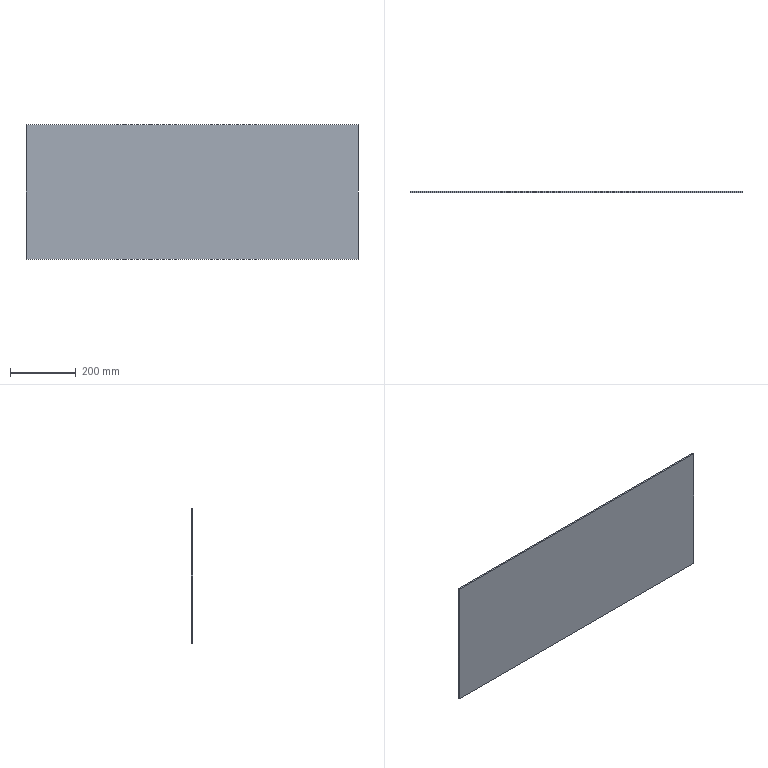Part | STEP file | door panel | 1 solid | 6 faces | box 1012 x 5 x 409 mm | volume 2069540 mm3 | plane 6
STEP:
#1=CARTESIAN_POINT('',(0.,0.,0.));
#2=DIRECTION('',(0.,0.,1.));
#3=DIRECTION('',(1.,0.,0.));
#4=AXIS2_PLACEMENT_3D('',#1,#2,#3);
#5=CARTESIAN_POINT('',(-506.,0.,-204.5));
#6=VERTEX_POINT('',#5);
#7=CARTESIAN_POINT('',(-506.,0.,204.5));
#8=VERTEX_POINT('',#7);
#9=CARTESIAN_POINT('',(-506.,0.,204.5));
#10=DIRECTION('',(0.,0.,1.));
#11=VECTOR('',#10,1.);
#12=LINE('',#9,#11);
#13=CARTESIAN_POINT('',(-506.,5.,204.5));
#14=DIRECTION('',(1.,0.,0.));
#15=DIRECTION('',(0.,0.,-1.));
#16=AXIS2_PLACEMENT_3D('',#13,#14,#15);
#17=PLANE('',#16);
#18=CARTESIAN_POINT('',(0.,-5.));
#19=DIRECTION('',(-1.,0.));
#20=VECTOR('',#19,1.);
#21=LINE('',#18,#20);
#22=(GEOMETRIC_REPRESENTATION_CONTEXT(2)PARAMETRIC_REPRESENTATION_CONTEXT()REPRESENTATION_CONTEXT('',''));
#23=DEFINITIONAL_REPRESENTATION('',(#21),#22);
#24=PCURVE('',#17,#23);
#25=CARTESIAN_POINT('',(0.,0.,0.));
#26=DIRECTION('',(0.,1.,0.));
#27=DIRECTION('',(0.,0.,1.));
#28=AXIS2_PLACEMENT_3D('',#25,#26,#27);
#29=PLANE('',#28);
#30=CARTESIAN_POINT('',(204.5,-506.));
#31=DIRECTION('',(1.,0.));
#32=VECTOR('',#31,1.);
#33=LINE('',#30,#32);
#34=(GEOMETRIC_REPRESENTATION_CONTEXT(2)PARAMETRIC_REPRESENTATION_CONTEXT()REPRESENTATION_CONTEXT('',''));
#35=DEFINITIONAL_REPRESENTATION('',(#33),#34);
#36=PCURVE('',#29,#35);
#37=SURFACE_CURVE('',#12,(#24,#36),.PCURVE_S1.);
#38=EDGE_CURVE('',#6,#8,#37,.T.);
#39=ORIENTED_EDGE('',*,*,#38,.T.);
#40=CARTESIAN_POINT('',(-506.,5.,204.5));
#41=VERTEX_POINT('',#40);
#42=CARTESIAN_POINT('',(-506.,5.,204.5));
#43=DIRECTION('',(0.,-1.,0.));
#44=VECTOR('',#43,1.);
#45=LINE('',#42,#44);
#46=CARTESIAN_POINT('',(0.,0.));
#47=DIRECTION('',(0.,-1.));
#48=VECTOR('',#47,1.);
#49=LINE('',#46,#48);
#50=(GEOMETRIC_REPRESENTATION_CONTEXT(2)PARAMETRIC_REPRESENTATION_CONTEXT()REPRESENTATION_CONTEXT('',''));
#51=DEFINITIONAL_REPRESENTATION('',(#49),#50);
#52=PCURVE('',#17,#51);
#53=CARTESIAN_POINT('',(506.,5.,204.5));
#54=DIRECTION('',(0.,0.,-1.));
#55=DIRECTION('',(-1.,0.,0.));
#56=AXIS2_PLACEMENT_3D('',#53,#54,#55);
#57=PLANE('',#56);
#58=CARTESIAN_POINT('',(1012.,0.));
#59=DIRECTION('',(0.,-1.));
#60=VECTOR('',#59,1.);
#61=LINE('',#58,#60);
#62=(GEOMETRIC_REPRESENTATION_CONTEXT(2)PARAMETRIC_REPRESENTATION_CONTEXT()REPRESENTATION_CONTEXT('',''));
#63=DEFINITIONAL_REPRESENTATION('',(#61),#62);
#64=PCURVE('',#57,#63);
#65=SURFACE_CURVE('',#45,(#52,#64),.PCURVE_S1.);
#66=EDGE_CURVE('',#41,#8,#65,.T.);
#67=ORIENTED_EDGE('',*,*,#66,.F.);
#68=CARTESIAN_POINT('',(-506.,5.,-204.5));
#69=VERTEX_POINT('',#68);
#70=CARTESIAN_POINT('',(-506.,5.,204.5));
#71=DIRECTION('',(0.,0.,1.));
#72=VECTOR('',#71,1.);
#73=LINE('',#70,#72);
#74=CARTESIAN_POINT('',(0.,0.));
#75=DIRECTION('',(-1.,0.));
#76=VECTOR('',#75,1.);
#77=LINE('',#74,#76);
#78=(GEOMETRIC_REPRESENTATION_CONTEXT(2)PARAMETRIC_REPRESENTATION_CONTEXT()REPRESENTATION_CONTEXT('',''));
#79=DEFINITIONAL_REPRESENTATION('',(#77),#78);
#80=PCURVE('',#17,#79);
#81=CARTESIAN_POINT('',(0.,5.,0.));
#82=DIRECTION('',(0.,1.,0.));
#83=DIRECTION('',(0.,0.,1.));
#84=AXIS2_PLACEMENT_3D('',#81,#82,#83);
#85=PLANE('',#84);
#86=CARTESIAN_POINT('',(204.5,-506.));
#87=DIRECTION('',(1.,0.));
#88=VECTOR('',#87,1.);
#89=LINE('',#86,#88);
#90=(GEOMETRIC_REPRESENTATION_CONTEXT(2)PARAMETRIC_REPRESENTATION_CONTEXT()REPRESENTATION_CONTEXT('',''));
#91=DEFINITIONAL_REPRESENTATION('',(#89),#90);
#92=PCURVE('',#85,#91);
#93=SURFACE_CURVE('',#73,(#80,#92),.PCURVE_S1.);
#94=EDGE_CURVE('',#69,#41,#93,.T.);
#95=ORIENTED_EDGE('',*,*,#94,.F.);
#96=CARTESIAN_POINT('',(-506.,5.,-204.5));
#97=DIRECTION('',(0.,-1.,0.));
#98=VECTOR('',#97,1.);
#99=LINE('',#96,#98);
#100=CARTESIAN_POINT('',(409.,0.));
#101=DIRECTION('',(0.,-1.));
#102=VECTOR('',#101,1.);
#103=LINE('',#100,#102);
#104=(GEOMETRIC_REPRESENTATION_CONTEXT(2)PARAMETRIC_REPRESENTATION_CONTEXT()REPRESENTATION_CONTEXT('',''));
#105=DEFINITIONAL_REPRESENTATION('',(#103),#104);
#106=PCURVE('',#17,#105);
#107=CARTESIAN_POINT('',(506.,5.,-204.5));
#108=DIRECTION('',(0.,0.,1.));
#109=DIRECTION('',(1.,0.,0.));
#110=AXIS2_PLACEMENT_3D('',#107,#108,#109);
#111=PLANE('',#110);
#112=CARTESIAN_POINT('',(-1012.,0.));
#113=DIRECTION('',(0.,-1.));
#114=VECTOR('',#113,1.);
#115=LINE('',#112,#114);
#116=(GEOMETRIC_REPRESENTATION_CONTEXT(2)PARAMETRIC_REPRESENTATION_CONTEXT()REPRESENTATION_CONTEXT('',''));
#117=DEFINITIONAL_REPRESENTATION('',(#115),#116);
#118=PCURVE('',#111,#117);
#119=SURFACE_CURVE('',#99,(#106,#118),.PCURVE_S1.);
#120=EDGE_CURVE('',#69,#6,#119,.T.);
#121=ORIENTED_EDGE('',*,*,#120,.T.);
#122=EDGE_LOOP('',(#39,#67,#95,#121));
#123=FACE_BOUND('',#122,.T.);
#124=ADVANCED_FACE('',(#123),#17,.F.);
#125=CARTESIAN_POINT('',(506.,0.,204.5));
#126=VERTEX_POINT('',#125);
#127=CARTESIAN_POINT('',(506.,0.,204.5));
#128=DIRECTION('',(1.,0.,0.));
#129=VECTOR('',#128,1.);
#130=LINE('',#127,#129);
#131=CARTESIAN_POINT('',(0.,-5.));
#132=DIRECTION('',(-1.,0.));
#133=VECTOR('',#132,1.);
#134=LINE('',#131,#133);
#135=(GEOMETRIC_REPRESENTATION_CONTEXT(2)PARAMETRIC_REPRESENTATION_CONTEXT()REPRESENTATION_CONTEXT('',''));
#136=DEFINITIONAL_REPRESENTATION('',(#134),#135);
#137=PCURVE('',#57,#136);
#138=CARTESIAN_POINT('',(204.5,506.));
#139=DIRECTION('',(0.,1.));
#140=VECTOR('',#139,1.);
#141=LINE('',#138,#140);
#142=(GEOMETRIC_REPRESENTATION_CONTEXT(2)PARAMETRIC_REPRESENTATION_CONTEXT()REPRESENTATION_CONTEXT('',''));
#143=DEFINITIONAL_REPRESENTATION('',(#141),#142);
#144=PCURVE('',#29,#143);
#145=SURFACE_CURVE('',#130,(#137,#144),.PCURVE_S1.);
#146=EDGE_CURVE('',#8,#126,#145,.T.);
#147=ORIENTED_EDGE('',*,*,#146,.T.);
#148=CARTESIAN_POINT('',(506.,5.,204.5));
#149=VERTEX_POINT('',#148);
#150=CARTESIAN_POINT('',(506.,5.,204.5));
#151=DIRECTION('',(0.,-1.,0.));
#152=VECTOR('',#151,1.);
#153=LINE('',#150,#152);
#154=CARTESIAN_POINT('',(0.,0.));
#155=DIRECTION('',(0.,-1.));
#156=VECTOR('',#155,1.);
#157=LINE('',#154,#156);
#158=(GEOMETRIC_REPRESENTATION_CONTEXT(2)PARAMETRIC_REPRESENTATION_CONTEXT()REPRESENTATION_CONTEXT('',''));
#159=DEFINITIONAL_REPRESENTATION('',(#157),#158);
#160=PCURVE('',#57,#159);
#161=CARTESIAN_POINT('',(506.,5.,204.5));
#162=DIRECTION('',(-1.,0.,0.));
#163=DIRECTION('',(0.,0.,1.));
#164=AXIS2_PLACEMENT_3D('',#161,#162,#163);
#165=PLANE('',#164);
#166=CARTESIAN_POINT('',(0.,0.));
#167=DIRECTION('',(0.,-1.));
#168=VECTOR('',#167,1.);
#169=LINE('',#166,#168);
#170=(GEOMETRIC_REPRESENTATION_CONTEXT(2)PARAMETRIC_REPRESENTATION_CONTEXT()REPRESENTATION_CONTEXT('',''));
#171=DEFINITIONAL_REPRESENTATION('',(#169),#170);
#172=PCURVE('',#165,#171);
#173=SURFACE_CURVE('',#153,(#160,#172),.PCURVE_S1.);
#174=EDGE_CURVE('',#149,#126,#173,.T.);
#175=ORIENTED_EDGE('',*,*,#174,.F.);
#176=CARTESIAN_POINT('',(506.,5.,204.5));
#177=DIRECTION('',(1.,0.,0.));
#178=VECTOR('',#177,1.);
#179=LINE('',#176,#178);
#180=CARTESIAN_POINT('',(0.,0.));
#181=DIRECTION('',(-1.,0.));
#182=VECTOR('',#181,1.);
#183=LINE('',#180,#182);
#184=(GEOMETRIC_REPRESENTATION_CONTEXT(2)PARAMETRIC_REPRESENTATION_CONTEXT()REPRESENTATION_CONTEXT('',''));
#185=DEFINITIONAL_REPRESENTATION('',(#183),#184);
#186=PCURVE('',#57,#185);
#187=CARTESIAN_POINT('',(204.5,506.));
#188=DIRECTION('',(0.,1.));
#189=VECTOR('',#188,1.);
#190=LINE('',#187,#189);
#191=(GEOMETRIC_REPRESENTATION_CONTEXT(2)PARAMETRIC_REPRESENTATION_CONTEXT()REPRESENTATION_CONTEXT('',''));
#192=DEFINITIONAL_REPRESENTATION('',(#190),#191);
#193=PCURVE('',#85,#192);
#194=SURFACE_CURVE('',#179,(#186,#193),.PCURVE_S1.);
#195=EDGE_CURVE('',#41,#149,#194,.T.);
#196=ORIENTED_EDGE('',*,*,#195,.F.);
#197=ORIENTED_EDGE('',*,*,#66,.T.);
#198=EDGE_LOOP('',(#147,#175,#196,#197));
#199=FACE_BOUND('',#198,.T.);
#200=ADVANCED_FACE('',(#199),#57,.F.);
#201=CARTESIAN_POINT('',(506.,0.,-204.5));
#202=VERTEX_POINT('',#201);
#203=CARTESIAN_POINT('',(506.,0.,204.5));
#204=DIRECTION('',(0.,0.,-1.));
#205=VECTOR('',#204,1.);
#206=LINE('',#203,#205);
#207=CARTESIAN_POINT('',(0.,-5.));
#208=DIRECTION('',(-1.,0.));
#209=VECTOR('',#208,1.);
#210=LINE('',#207,#209);
#211=(GEOMETRIC_REPRESENTATION_CONTEXT(2)PARAMETRIC_REPRESENTATION_CONTEXT()REPRESENTATION_CONTEXT('',''));
#212=DEFINITIONAL_REPRESENTATION('',(#210),#211);
#213=PCURVE('',#165,#212);
#214=CARTESIAN_POINT('',(204.5,506.));
#215=DIRECTION('',(-1.,0.));
#216=VECTOR('',#215,1.);
#217=LINE('',#214,#216);
#218=(GEOMETRIC_REPRESENTATION_CONTEXT(2)PARAMETRIC_REPRESENTATION_CONTEXT()REPRESENTATION_CONTEXT('',''));
#219=DEFINITIONAL_REPRESENTATION('',(#217),#218);
#220=PCURVE('',#29,#219);
#221=SURFACE_CURVE('',#206,(#213,#220),.PCURVE_S1.);
#222=EDGE_CURVE('',#126,#202,#221,.T.);
#223=ORIENTED_EDGE('',*,*,#222,.T.);
#224=CARTESIAN_POINT('',(506.,5.,-204.5));
#225=VERTEX_POINT('',#224);
#226=CARTESIAN_POINT('',(506.,5.,-204.5));
#227=DIRECTION('',(0.,-1.,0.));
#228=VECTOR('',#227,1.);
#229=LINE('',#226,#228);
#230=CARTESIAN_POINT('',(-409.,0.));
#231=DIRECTION('',(0.,-1.));
#232=VECTOR('',#231,1.);
#233=LINE('',#230,#232);
#234=(GEOMETRIC_REPRESENTATION_CONTEXT(2)PARAMETRIC_REPRESENTATION_CONTEXT()REPRESENTATION_CONTEXT('',''));
#235=DEFINITIONAL_REPRESENTATION('',(#233),#234);
#236=PCURVE('',#165,#235);
#237=CARTESIAN_POINT('',(0.,0.));
#238=DIRECTION('',(0.,-1.));
#239=VECTOR('',#238,1.);
#240=LINE('',#237,#239);
#241=(GEOMETRIC_REPRESENTATION_CONTEXT(2)PARAMETRIC_REPRESENTATION_CONTEXT()REPRESENTATION_CONTEXT('',''));
#242=DEFINITIONAL_REPRESENTATION('',(#240),#241);
#243=PCURVE('',#111,#242);
#244=SURFACE_CURVE('',#229,(#236,#243),.PCURVE_S1.);
#245=EDGE_CURVE('',#225,#202,#244,.T.);
#246=ORIENTED_EDGE('',*,*,#245,.F.);
#247=CARTESIAN_POINT('',(506.,5.,204.5));
#248=DIRECTION('',(0.,0.,-1.));
#249=VECTOR('',#248,1.);
#250=LINE('',#247,#249);
#251=CARTESIAN_POINT('',(0.,0.));
#252=DIRECTION('',(-1.,0.));
#253=VECTOR('',#252,1.);
#254=LINE('',#251,#253);
#255=(GEOMETRIC_REPRESENTATION_CONTEXT(2)PARAMETRIC_REPRESENTATION_CONTEXT()REPRESENTATION_CONTEXT('',''));
#256=DEFINITIONAL_REPRESENTATION('',(#254),#255);
#257=PCURVE('',#165,#256);
#258=CARTESIAN_POINT('',(204.5,506.));
#259=DIRECTION('',(-1.,0.));
#260=VECTOR('',#259,1.);
#261=LINE('',#258,#260);
#262=(GEOMETRIC_REPRESENTATION_CONTEXT(2)PARAMETRIC_REPRESENTATION_CONTEXT()REPRESENTATION_CONTEXT('',''));
#263=DEFINITIONAL_REPRESENTATION('',(#261),#262);
#264=PCURVE('',#85,#263);
#265=SURFACE_CURVE('',#250,(#257,#264),.PCURVE_S1.);
#266=EDGE_CURVE('',#149,#225,#265,.T.);
#267=ORIENTED_EDGE('',*,*,#266,.F.);
#268=ORIENTED_EDGE('',*,*,#174,.T.);
#269=EDGE_LOOP('',(#223,#246,#267,#268));
#270=FACE_BOUND('',#269,.T.);
#271=ADVANCED_FACE('',(#270),#165,.F.);
#272=CARTESIAN_POINT('',(506.,0.,-204.5));
#273=DIRECTION('',(-1.,0.,0.));
#274=VECTOR('',#273,1.);
#275=LINE('',#272,#274);
#276=CARTESIAN_POINT('',(0.,-5.));
#277=DIRECTION('',(-1.,0.));
#278=VECTOR('',#277,1.);
#279=LINE('',#276,#278);
#280=(GEOMETRIC_REPRESENTATION_CONTEXT(2)PARAMETRIC_REPRESENTATION_CONTEXT()REPRESENTATION_CONTEXT('',''));
#281=DEFINITIONAL_REPRESENTATION('',(#279),#280);
#282=PCURVE('',#111,#281);
#283=CARTESIAN_POINT('',(-204.5,506.));
#284=DIRECTION('',(0.,-1.));
#285=VECTOR('',#284,1.);
#286=LINE('',#283,#285);
#287=(GEOMETRIC_REPRESENTATION_CONTEXT(2)PARAMETRIC_REPRESENTATION_CONTEXT()REPRESENTATION_CONTEXT('',''));
#288=DEFINITIONAL_REPRESENTATION('',(#286),#287);
#289=PCURVE('',#29,#288);
#290=SURFACE_CURVE('',#275,(#282,#289),.PCURVE_S1.);
#291=EDGE_CURVE('',#202,#6,#290,.T.);
#292=ORIENTED_EDGE('',*,*,#291,.T.);
#293=ORIENTED_EDGE('',*,*,#120,.F.);
#294=CARTESIAN_POINT('',(506.,5.,-204.5));
#295=DIRECTION('',(-1.,0.,0.));
#296=VECTOR('',#295,1.);
#297=LINE('',#294,#296);
#298=CARTESIAN_POINT('',(0.,0.));
#299=DIRECTION('',(-1.,0.));
#300=VECTOR('',#299,1.);
#301=LINE('',#298,#300);
#302=(GEOMETRIC_REPRESENTATION_CONTEXT(2)PARAMETRIC_REPRESENTATION_CONTEXT()REPRESENTATION_CONTEXT('',''));
#303=DEFINITIONAL_REPRESENTATION('',(#301),#302);
#304=PCURVE('',#111,#303);
#305=CARTESIAN_POINT('',(-204.5,506.));
#306=DIRECTION('',(0.,-1.));
#307=VECTOR('',#306,1.);
#308=LINE('',#305,#307);
#309=(GEOMETRIC_REPRESENTATION_CONTEXT(2)PARAMETRIC_REPRESENTATION_CONTEXT()REPRESENTATION_CONTEXT('',''));
#310=DEFINITIONAL_REPRESENTATION('',(#308),#309);
#311=PCURVE('',#85,#310);
#312=SURFACE_CURVE('',#297,(#304,#311),.PCURVE_S1.);
#313=EDGE_CURVE('',#225,#69,#312,.T.);
#314=ORIENTED_EDGE('',*,*,#313,.F.);
#315=ORIENTED_EDGE('',*,*,#245,.T.);
#316=EDGE_LOOP('',(#292,#293,#314,#315));
#317=FACE_BOUND('',#316,.T.);
#318=ADVANCED_FACE('',(#317),#111,.F.);
#319=ORIENTED_EDGE('',*,*,#94,.T.);
#320=ORIENTED_EDGE('',*,*,#195,.T.);
#321=ORIENTED_EDGE('',*,*,#266,.T.);
#322=ORIENTED_EDGE('',*,*,#313,.T.);
#323=EDGE_LOOP('',(#319,#320,#321,#322));
#324=FACE_BOUND('',#323,.T.);
#325=ADVANCED_FACE('',(#324),#85,.T.);
#326=ORIENTED_EDGE('',*,*,#38,.F.);
#327=ORIENTED_EDGE('',*,*,#291,.F.);
#328=ORIENTED_EDGE('',*,*,#222,.F.);
#329=ORIENTED_EDGE('',*,*,#146,.F.);
#330=EDGE_LOOP('',(#326,#327,#328,#329));
#331=FACE_BOUND('',#330,.T.);
#332=ADVANCED_FACE('',(#331),#29,.F.);
#333=CLOSED_SHELL('',(#124,#200,#271,#318,#325,#332));
#334=MANIFOLD_SOLID_BREP('',#333);
#335=(LENGTH_UNIT()NAMED_UNIT(*)SI_UNIT(.MILLI.,.METRE.));
#336=UNCERTAINTY_MEASURE_WITH_UNIT(LENGTH_MEASURE(0.0000001),#335,'','');
#337=(NAMED_UNIT(*)PLANE_ANGLE_UNIT()SI_UNIT($,.RADIAN.));
#338=(NAMED_UNIT(*)SI_UNIT($,.STERADIAN.)SOLID_ANGLE_UNIT());
#339=(GEOMETRIC_REPRESENTATION_CONTEXT(3)GLOBAL_UNCERTAINTY_ASSIGNED_CONTEXT((#336))GLOBAL_UNIT_ASSIGNED_CONTEXT((#335,#337,#338))REPRESENTATION_CONTEXT('',''));
#340=ADVANCED_BREP_SHAPE_REPRESENTATION('',(#4,#334),#339);